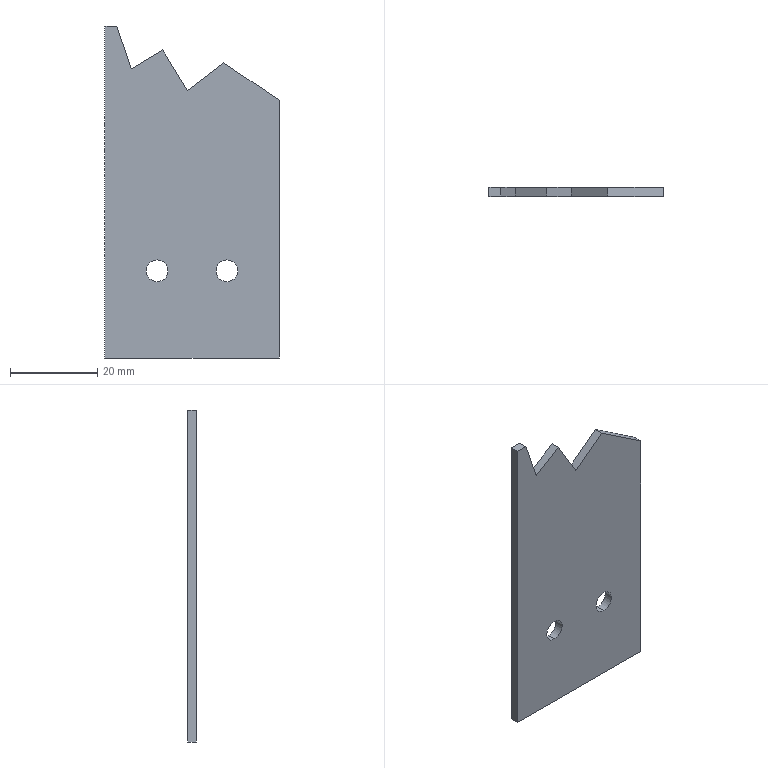Part | SolidWorks | features Cut 2, Extrusion 1 | 1 solid | 15 faces | box 40 x 2 x 76.221 mm | volume 5242 mm3 | plane 11 | cylinder 4 | commonest cylinder face diameters 5 x4
STEP:
#1=CARTESIAN_POINT('',(8.,2.,-22.5));
#2=VERTEX_POINT('',#1);
#3=CARTESIAN_POINT('',(8.,2.,-17.5));
#4=VERTEX_POINT('',#3);
#5=CARTESIAN_POINT('',(8.,2.,-20.));
#6=DIRECTION('',(0.,1.,0.));
#7=DIRECTION('',(0.,0.,1.));
#8=AXIS2_PLACEMENT_3D('',#5,#6,#7);
#9=CIRCLE('',#8,2.5);
#10=EDGE_CURVE('',#2,#4,#9,.T.);
#11=ORIENTED_EDGE('',*,*,#10,.T.);
#12=CARTESIAN_POINT('',(8.,0.,-17.5));
#13=VERTEX_POINT('',#12);
#14=CARTESIAN_POINT('',(8.,10.,-17.5));
#15=DIRECTION('',(0.,-1.,0.));
#16=VECTOR('',#15,1000.);
#17=LINE('',#14,#16);
#18=EDGE_CURVE('',#4,#13,#17,.T.);
#19=ORIENTED_EDGE('',*,*,#18,.T.);
#20=CARTESIAN_POINT('',(8.,0.,-22.5));
#21=VERTEX_POINT('',#20);
#22=CARTESIAN_POINT('',(8.,0.,-20.));
#23=DIRECTION('',(0.,-1.,0.));
#24=DIRECTION('',(0.,0.,-1.));
#25=AXIS2_PLACEMENT_3D('',#22,#23,#24);
#26=CIRCLE('',#25,2.5);
#27=EDGE_CURVE('',#13,#21,#26,.T.);
#28=ORIENTED_EDGE('',*,*,#27,.T.);
#29=CARTESIAN_POINT('',(8.,10.,-22.5));
#30=DIRECTION('',(0.,-1.,0.));
#31=VECTOR('',#30,1000.);
#32=LINE('',#29,#31);
#33=EDGE_CURVE('',#2,#21,#32,.T.);
#34=ORIENTED_EDGE('',*,*,#33,.F.);
#35=EDGE_LOOP('',(#11,#19,#28,#34));
#36=FACE_OUTER_BOUND('',#35,.T.);
#37=CARTESIAN_POINT('',(8.,10.,-20.));
#38=DIRECTION('',(0.,-1.,0.));
#39=DIRECTION('',(0.,0.,-1.));
#40=AXIS2_PLACEMENT_3D('',#37,#38,#39);
#41=CYLINDRICAL_SURFACE('',#40,2.5);
#42=ADVANCED_FACE('',(#36),#41,.F.);
#43=CARTESIAN_POINT('',(-8.,2.,-22.5));
#44=VERTEX_POINT('',#43);
#45=CARTESIAN_POINT('',(-8.,2.,-17.5));
#46=VERTEX_POINT('',#45);
#47=CARTESIAN_POINT('',(-8.,2.,-20.));
#48=DIRECTION('',(0.,1.,0.));
#49=DIRECTION('',(0.,0.,1.));
#50=AXIS2_PLACEMENT_3D('',#47,#48,#49);
#51=CIRCLE('',#50,2.5);
#52=EDGE_CURVE('',#44,#46,#51,.T.);
#53=ORIENTED_EDGE('',*,*,#52,.T.);
#54=CARTESIAN_POINT('',(-8.,0.,-17.5));
#55=VERTEX_POINT('',#54);
#56=CARTESIAN_POINT('',(-8.,10.,-17.5));
#57=DIRECTION('',(0.,-1.,0.));
#58=VECTOR('',#57,1000.);
#59=LINE('',#56,#58);
#60=EDGE_CURVE('',#46,#55,#59,.T.);
#61=ORIENTED_EDGE('',*,*,#60,.T.);
#62=CARTESIAN_POINT('',(-8.,0.,-22.5));
#63=VERTEX_POINT('',#62);
#64=CARTESIAN_POINT('',(-8.,0.,-20.));
#65=DIRECTION('',(0.,-1.,0.));
#66=DIRECTION('',(0.,0.,-1.));
#67=AXIS2_PLACEMENT_3D('',#64,#65,#66);
#68=CIRCLE('',#67,2.5);
#69=EDGE_CURVE('',#55,#63,#68,.T.);
#70=ORIENTED_EDGE('',*,*,#69,.T.);
#71=CARTESIAN_POINT('',(-8.,10.,-22.5));
#72=DIRECTION('',(0.,-1.,0.));
#73=VECTOR('',#72,1000.);
#74=LINE('',#71,#73);
#75=EDGE_CURVE('',#44,#63,#74,.T.);
#76=ORIENTED_EDGE('',*,*,#75,.F.);
#77=EDGE_LOOP('',(#53,#61,#70,#76));
#78=FACE_OUTER_BOUND('',#77,.T.);
#79=CARTESIAN_POINT('',(-8.,10.,-20.));
#80=DIRECTION('',(0.,-1.,0.));
#81=DIRECTION('',(0.,0.,-1.));
#82=AXIS2_PLACEMENT_3D('',#79,#80,#81);
#83=CYLINDRICAL_SURFACE('',#82,2.5);
#84=ADVANCED_FACE('',(#78),#83,.F.);
#85=CARTESIAN_POINT('',(20.,2.,19.198));
#86=VERTEX_POINT('',#85);
#87=CARTESIAN_POINT('',(20.,2.,-40.));
#88=VERTEX_POINT('',#87);
#89=CARTESIAN_POINT('',(20.,2.,-40.));
#90=DIRECTION('',(0.,0.,-1.));
#91=VECTOR('',#90,1000.);
#92=LINE('',#89,#91);
#93=EDGE_CURVE('',#86,#88,#92,.T.);
#94=ORIENTED_EDGE('',*,*,#93,.F.);
#95=CARTESIAN_POINT('',(20.,0.,19.198));
#96=VERTEX_POINT('',#95);
#97=CARTESIAN_POINT('',(20.,-8.,19.198));
#98=DIRECTION('',(0.,1.,0.));
#99=VECTOR('',#98,1000.);
#100=LINE('',#97,#99);
#101=EDGE_CURVE('',#96,#86,#100,.T.);
#102=ORIENTED_EDGE('',*,*,#101,.F.);
#103=CARTESIAN_POINT('',(20.,0.,-40.));
#104=VERTEX_POINT('',#103);
#105=CARTESIAN_POINT('',(20.,0.,-40.));
#106=DIRECTION('',(0.,0.,-1.));
#107=VECTOR('',#106,1000.);
#108=LINE('',#105,#107);
#109=EDGE_CURVE('',#96,#104,#108,.T.);
#110=ORIENTED_EDGE('',*,*,#109,.T.);
#111=CARTESIAN_POINT('',(20.,2.,-40.));
#112=DIRECTION('',(0.,-1.,0.));
#113=VECTOR('',#112,1000.);
#114=LINE('',#111,#113);
#115=EDGE_CURVE('',#88,#104,#114,.T.);
#116=ORIENTED_EDGE('',*,*,#115,.F.);
#117=EDGE_LOOP('',(#94,#102,#110,#116));
#118=FACE_OUTER_BOUND('',#117,.T.);
#119=CARTESIAN_POINT('',(20.,2.,-40.));
#120=DIRECTION('',(-1.,0.,0.));
#121=DIRECTION('',(0.,0.,1.));
#122=AXIS2_PLACEMENT_3D('',#119,#120,#121);
#123=PLANE('',#122);
#124=ADVANCED_FACE('',(#118),#123,.F.);
#125=CARTESIAN_POINT('',(-20.,0.,-40.));
#126=VERTEX_POINT('',#125);
#127=CARTESIAN_POINT('',(-20.,0.,-40.));
#128=DIRECTION('',(-1.,0.,0.));
#129=VECTOR('',#128,1000.);
#130=LINE('',#127,#129);
#131=EDGE_CURVE('',#104,#126,#130,.T.);
#132=ORIENTED_EDGE('',*,*,#131,.T.);
#133=CARTESIAN_POINT('',(-20.,2.,-40.));
#134=VERTEX_POINT('',#133);
#135=CARTESIAN_POINT('',(-20.,2.,-40.));
#136=DIRECTION('',(0.,-1.,0.));
#137=VECTOR('',#136,1000.);
#138=LINE('',#135,#137);
#139=EDGE_CURVE('',#134,#126,#138,.T.);
#140=ORIENTED_EDGE('',*,*,#139,.F.);
#141=CARTESIAN_POINT('',(-20.,2.,-40.));
#142=DIRECTION('',(-1.,0.,0.));
#143=VECTOR('',#142,1000.);
#144=LINE('',#141,#143);
#145=EDGE_CURVE('',#88,#134,#144,.T.);
#146=ORIENTED_EDGE('',*,*,#145,.F.);
#147=ORIENTED_EDGE('',*,*,#115,.T.);
#148=EDGE_LOOP('',(#132,#140,#146,#147));
#149=FACE_OUTER_BOUND('',#148,.T.);
#150=CARTESIAN_POINT('',(-20.,2.,-40.));
#151=DIRECTION('',(0.,0.,1.));
#152=DIRECTION('',(1.,0.,0.));
#153=AXIS2_PLACEMENT_3D('',#150,#151,#152);
#154=PLANE('',#153);
#155=ADVANCED_FACE('',(#149),#154,.F.);
#156=CARTESIAN_POINT('',(-20.,0.,36.221));
#157=VERTEX_POINT('',#156);
#158=CARTESIAN_POINT('',(-20.,0.,-40.));
#159=DIRECTION('',(0.,0.,1.));
#160=VECTOR('',#159,1000.);
#161=LINE('',#158,#160);
#162=EDGE_CURVE('',#126,#157,#161,.T.);
#163=ORIENTED_EDGE('',*,*,#162,.T.);
#164=CARTESIAN_POINT('',(-20.,2.,36.221));
#165=VERTEX_POINT('',#164);
#166=CARTESIAN_POINT('',(-20.,-8.,36.221));
#167=DIRECTION('',(0.,1.,0.));
#168=VECTOR('',#167,1000.);
#169=LINE('',#166,#168);
#170=EDGE_CURVE('',#157,#165,#169,.T.);
#171=ORIENTED_EDGE('',*,*,#170,.T.);
#172=CARTESIAN_POINT('',(-20.,2.,-40.));
#173=DIRECTION('',(0.,0.,1.));
#174=VECTOR('',#173,1000.);
#175=LINE('',#172,#174);
#176=EDGE_CURVE('',#134,#165,#175,.T.);
#177=ORIENTED_EDGE('',*,*,#176,.F.);
#178=ORIENTED_EDGE('',*,*,#139,.T.);
#179=EDGE_LOOP('',(#163,#171,#177,#178));
#180=FACE_OUTER_BOUND('',#179,.T.);
#181=CARTESIAN_POINT('',(-20.,2.,-40.));
#182=DIRECTION('',(1.,0.,0.));
#183=DIRECTION('',(0.,0.,-1.));
#184=AXIS2_PLACEMENT_3D('',#181,#182,#183);
#185=PLANE('',#184);
#186=ADVANCED_FACE('',(#180),#185,.F.);
#187=CARTESIAN_POINT('',(-17.266,2.,36.221));
#188=VERTEX_POINT('',#187);
#189=CARTESIAN_POINT('',(-17.266,2.,36.221));
#190=DIRECTION('',(-1.,0.,0.));
#191=VECTOR('',#190,1000.);
#192=LINE('',#189,#191);
#193=EDGE_CURVE('',#188,#165,#192,.T.);
#194=ORIENTED_EDGE('',*,*,#193,.F.);
#195=CARTESIAN_POINT('',(-13.941,2.,26.358));
#196=VERTEX_POINT('',#195);
#197=CARTESIAN_POINT('',(-13.941,2.,26.358));
#198=DIRECTION('',(-0.3194,0.,0.9476));
#199=VECTOR('',#198,1000.);
#200=LINE('',#197,#199);
#201=EDGE_CURVE('',#196,#188,#200,.T.);
#202=ORIENTED_EDGE('',*,*,#201,.F.);
#203=CARTESIAN_POINT('',(-6.728,2.,30.727));
#204=VERTEX_POINT('',#203);
#205=CARTESIAN_POINT('',(-6.728,2.,30.727));
#206=DIRECTION('',(-0.8553,0.,-0.5181));
#207=VECTOR('',#206,1000.);
#208=LINE('',#205,#207);
#209=EDGE_CURVE('',#204,#196,#208,.T.);
#210=ORIENTED_EDGE('',*,*,#209,.F.);
#211=CARTESIAN_POINT('',(-1.054,2.,21.36));
#212=VERTEX_POINT('',#211);
#213=CARTESIAN_POINT('',(-1.054,2.,21.36));
#214=DIRECTION('',(-0.5181,0.,0.8553));
#215=VECTOR('',#214,1000.);
#216=LINE('',#213,#215);
#217=EDGE_CURVE('',#212,#204,#216,.T.);
#218=ORIENTED_EDGE('',*,*,#217,.F.);
#219=CARTESIAN_POINT('',(7.323,2.,27.755));
#220=VERTEX_POINT('',#219);
#221=CARTESIAN_POINT('',(7.323,2.,27.755));
#222=DIRECTION('',(-0.7948,0.,-0.6068));
#223=VECTOR('',#222,1000.);
#224=LINE('',#221,#223);
#225=EDGE_CURVE('',#220,#212,#224,.T.);
#226=ORIENTED_EDGE('',*,*,#225,.F.);
#227=CARTESIAN_POINT('',(20.,2.,19.198));
#228=DIRECTION('',(-0.8289,0.,0.5595));
#229=VECTOR('',#228,1000.);
#230=LINE('',#227,#229);
#231=EDGE_CURVE('',#86,#220,#230,.T.);
#232=ORIENTED_EDGE('',*,*,#231,.F.);
#233=ORIENTED_EDGE('',*,*,#93,.T.);
#234=ORIENTED_EDGE('',*,*,#145,.T.);
#235=ORIENTED_EDGE('',*,*,#176,.T.);
#236=EDGE_LOOP('',(#194,#202,#210,#218,#226,#232,#233,#234,#235));
#237=FACE_OUTER_BOUND('',#236,.T.);
#238=ORIENTED_EDGE('',*,*,#10,.F.);
#239=CARTESIAN_POINT('',(8.,2.,-20.));
#240=DIRECTION('',(0.,1.,0.));
#241=DIRECTION('',(0.,0.,1.));
#242=AXIS2_PLACEMENT_3D('',#239,#240,#241);
#243=CIRCLE('',#242,2.5);
#244=EDGE_CURVE('',#4,#2,#243,.T.);
#245=ORIENTED_EDGE('',*,*,#244,.F.);
#246=EDGE_LOOP('',(#238,#245));
#247=FACE_BOUND('',#246,.T.);
#248=ORIENTED_EDGE('',*,*,#52,.F.);
#249=CARTESIAN_POINT('',(-8.,2.,-20.));
#250=DIRECTION('',(0.,1.,0.));
#251=DIRECTION('',(0.,0.,1.));
#252=AXIS2_PLACEMENT_3D('',#249,#250,#251);
#253=CIRCLE('',#252,2.5);
#254=EDGE_CURVE('',#46,#44,#253,.T.);
#255=ORIENTED_EDGE('',*,*,#254,.F.);
#256=EDGE_LOOP('',(#248,#255));
#257=FACE_BOUND('',#256,.T.);
#258=CARTESIAN_POINT('',(0.,2.,0.));
#259=DIRECTION('',(0.,1.,0.));
#260=DIRECTION('',(0.,0.,1.));
#261=AXIS2_PLACEMENT_3D('',#258,#259,#260);
#262=PLANE('',#261);
#263=ADVANCED_FACE('',(#237,#247,#257),#262,.T.);
#264=CARTESIAN_POINT('',(8.,0.,-20.));
#265=DIRECTION('',(0.,-1.,0.));
#266=DIRECTION('',(0.,0.,-1.));
#267=AXIS2_PLACEMENT_3D('',#264,#265,#266);
#268=CIRCLE('',#267,2.5);
#269=EDGE_CURVE('',#21,#13,#268,.T.);
#270=ORIENTED_EDGE('',*,*,#269,.F.);
#271=ORIENTED_EDGE('',*,*,#27,.F.);
#272=EDGE_LOOP('',(#270,#271));
#273=FACE_BOUND('',#272,.T.);
#274=CARTESIAN_POINT('',(-8.,0.,-20.));
#275=DIRECTION('',(0.,-1.,0.));
#276=DIRECTION('',(0.,0.,-1.));
#277=AXIS2_PLACEMENT_3D('',#274,#275,#276);
#278=CIRCLE('',#277,2.5);
#279=EDGE_CURVE('',#63,#55,#278,.T.);
#280=ORIENTED_EDGE('',*,*,#279,.F.);
#281=ORIENTED_EDGE('',*,*,#69,.F.);
#282=EDGE_LOOP('',(#280,#281));
#283=FACE_BOUND('',#282,.T.);
#284=CARTESIAN_POINT('',(-13.941,0.,26.358));
#285=VERTEX_POINT('',#284);
#286=CARTESIAN_POINT('',(-17.266,0.,36.221));
#287=VERTEX_POINT('',#286);
#288=CARTESIAN_POINT('',(-4.54,0.,-1.53));
#289=DIRECTION('',(-0.3194,0.,0.9476));
#290=VECTOR('',#289,1000.);
#291=LINE('',#288,#290);
#292=EDGE_CURVE('',#285,#287,#291,.T.);
#293=ORIENTED_EDGE('',*,*,#292,.T.);
#294=CARTESIAN_POINT('',(0.,0.,36.221));
#295=DIRECTION('',(-1.,0.,0.));
#296=VECTOR('',#295,1000.);
#297=LINE('',#294,#296);
#298=EDGE_CURVE('',#287,#157,#297,.T.);
#299=ORIENTED_EDGE('',*,*,#298,.T.);
#300=ORIENTED_EDGE('',*,*,#162,.F.);
#301=ORIENTED_EDGE('',*,*,#131,.F.);
#302=ORIENTED_EDGE('',*,*,#109,.F.);
#303=CARTESIAN_POINT('',(7.323,0.,27.755));
#304=VERTEX_POINT('',#303);
#305=CARTESIAN_POINT('',(15.162,0.,22.464));
#306=DIRECTION('',(-0.8289,0.,0.5595));
#307=VECTOR('',#306,1000.);
#308=LINE('',#305,#307);
#309=EDGE_CURVE('',#96,#304,#308,.T.);
#310=ORIENTED_EDGE('',*,*,#309,.T.);
#311=CARTESIAN_POINT('',(-1.054,0.,21.36));
#312=VERTEX_POINT('',#311);
#313=CARTESIAN_POINT('',(-10.69,0.,14.003));
#314=DIRECTION('',(-0.7948,0.,-0.6068));
#315=VECTOR('',#314,1000.);
#316=LINE('',#313,#315);
#317=EDGE_CURVE('',#304,#312,#316,.T.);
#318=ORIENTED_EDGE('',*,*,#317,.T.);
#319=CARTESIAN_POINT('',(-6.728,0.,30.727));
#320=VERTEX_POINT('',#319);
#321=CARTESIAN_POINT('',(8.695,0.,5.267));
#322=DIRECTION('',(-0.5181,0.,0.8553));
#323=VECTOR('',#322,1000.);
#324=LINE('',#321,#323);
#325=EDGE_CURVE('',#312,#320,#324,.T.);
#326=ORIENTED_EDGE('',*,*,#325,.T.);
#327=CARTESIAN_POINT('',(-15.423,0.,25.46));
#328=DIRECTION('',(-0.8553,0.,-0.5181));
#329=VECTOR('',#328,1000.);
#330=LINE('',#327,#329);
#331=EDGE_CURVE('',#320,#285,#330,.T.);
#332=ORIENTED_EDGE('',*,*,#331,.T.);
#333=EDGE_LOOP('',(#293,#299,#300,#301,#302,#310,#318,#326,#332));
#334=FACE_OUTER_BOUND('',#333,.T.);
#335=CARTESIAN_POINT('',(0.,0.,0.));
#336=DIRECTION('',(0.,1.,0.));
#337=DIRECTION('',(0.,0.,1.));
#338=AXIS2_PLACEMENT_3D('',#335,#336,#337);
#339=PLANE('',#338);
#340=ADVANCED_FACE('',(#273,#283,#334),#339,.F.);
#341=ORIENTED_EDGE('',*,*,#60,.F.);
#342=ORIENTED_EDGE('',*,*,#254,.T.);
#343=ORIENTED_EDGE('',*,*,#75,.T.);
#344=ORIENTED_EDGE('',*,*,#279,.T.);
#345=EDGE_LOOP('',(#341,#342,#343,#344));
#346=FACE_OUTER_BOUND('',#345,.T.);
#347=CARTESIAN_POINT('',(-8.,10.,-20.));
#348=DIRECTION('',(0.,-1.,0.));
#349=DIRECTION('',(0.,0.,-1.));
#350=AXIS2_PLACEMENT_3D('',#347,#348,#349);
#351=CYLINDRICAL_SURFACE('',#350,2.5);
#352=ADVANCED_FACE('',(#346),#351,.F.);
#353=ORIENTED_EDGE('',*,*,#18,.F.);
#354=ORIENTED_EDGE('',*,*,#244,.T.);
#355=ORIENTED_EDGE('',*,*,#33,.T.);
#356=ORIENTED_EDGE('',*,*,#269,.T.);
#357=EDGE_LOOP('',(#353,#354,#355,#356));
#358=FACE_OUTER_BOUND('',#357,.T.);
#359=CARTESIAN_POINT('',(8.,10.,-20.));
#360=DIRECTION('',(0.,-1.,0.));
#361=DIRECTION('',(0.,0.,-1.));
#362=AXIS2_PLACEMENT_3D('',#359,#360,#361);
#363=CYLINDRICAL_SURFACE('',#362,2.5);
#364=ADVANCED_FACE('',(#358),#363,.F.);
#365=CARTESIAN_POINT('',(-17.266,-8.,36.221));
#366=DIRECTION('',(0.,1.,0.));
#367=VECTOR('',#366,1000.);
#368=LINE('',#365,#367);
#369=EDGE_CURVE('',#287,#188,#368,.T.);
#370=ORIENTED_EDGE('',*,*,#369,.T.);
#371=ORIENTED_EDGE('',*,*,#193,.T.);
#372=ORIENTED_EDGE('',*,*,#170,.F.);
#373=ORIENTED_EDGE('',*,*,#298,.F.);
#374=EDGE_LOOP('',(#370,#371,#372,#373));
#375=FACE_OUTER_BOUND('',#374,.T.);
#376=CARTESIAN_POINT('',(-17.266,-8.,36.221));
#377=DIRECTION('',(0.,0.,-1.));
#378=DIRECTION('',(-1.,0.,0.));
#379=AXIS2_PLACEMENT_3D('',#376,#377,#378);
#380=PLANE('',#379);
#381=ADVANCED_FACE('',(#375),#380,.F.);
#382=CARTESIAN_POINT('',(-13.941,-8.,26.358));
#383=DIRECTION('',(0.,1.,0.));
#384=VECTOR('',#383,1000.);
#385=LINE('',#382,#384);
#386=EDGE_CURVE('',#285,#196,#385,.T.);
#387=ORIENTED_EDGE('',*,*,#386,.T.);
#388=ORIENTED_EDGE('',*,*,#201,.T.);
#389=ORIENTED_EDGE('',*,*,#369,.F.);
#390=ORIENTED_EDGE('',*,*,#292,.F.);
#391=EDGE_LOOP('',(#387,#388,#389,#390));
#392=FACE_OUTER_BOUND('',#391,.T.);
#393=CARTESIAN_POINT('',(-13.941,-8.,26.358));
#394=DIRECTION('',(-0.9476,0.,-0.3194));
#395=DIRECTION('',(-0.3194,0.,0.9476));
#396=AXIS2_PLACEMENT_3D('',#393,#394,#395);
#397=PLANE('',#396);
#398=ADVANCED_FACE('',(#392),#397,.F.);
#399=CARTESIAN_POINT('',(-6.728,-8.,30.727));
#400=DIRECTION('',(0.,1.,0.));
#401=VECTOR('',#400,1000.);
#402=LINE('',#399,#401);
#403=EDGE_CURVE('',#320,#204,#402,.T.);
#404=ORIENTED_EDGE('',*,*,#403,.T.);
#405=ORIENTED_EDGE('',*,*,#209,.T.);
#406=ORIENTED_EDGE('',*,*,#386,.F.);
#407=ORIENTED_EDGE('',*,*,#331,.F.);
#408=EDGE_LOOP('',(#404,#405,#406,#407));
#409=FACE_OUTER_BOUND('',#408,.T.);
#410=CARTESIAN_POINT('',(-6.728,-8.,30.727));
#411=DIRECTION('',(0.5181,0.,-0.8553));
#412=DIRECTION('',(-0.8553,0.,-0.5181));
#413=AXIS2_PLACEMENT_3D('',#410,#411,#412);
#414=PLANE('',#413);
#415=ADVANCED_FACE('',(#409),#414,.F.);
#416=CARTESIAN_POINT('',(-1.054,-8.,21.36));
#417=DIRECTION('',(0.,1.,0.));
#418=VECTOR('',#417,1000.);
#419=LINE('',#416,#418);
#420=EDGE_CURVE('',#312,#212,#419,.T.);
#421=ORIENTED_EDGE('',*,*,#420,.T.);
#422=ORIENTED_EDGE('',*,*,#217,.T.);
#423=ORIENTED_EDGE('',*,*,#403,.F.);
#424=ORIENTED_EDGE('',*,*,#325,.F.);
#425=EDGE_LOOP('',(#421,#422,#423,#424));
#426=FACE_OUTER_BOUND('',#425,.T.);
#427=CARTESIAN_POINT('',(-1.054,-8.,21.36));
#428=DIRECTION('',(-0.8553,0.,-0.5181));
#429=DIRECTION('',(-0.5181,0.,0.8553));
#430=AXIS2_PLACEMENT_3D('',#427,#428,#429);
#431=PLANE('',#430);
#432=ADVANCED_FACE('',(#426),#431,.F.);
#433=CARTESIAN_POINT('',(7.323,-8.,27.755));
#434=DIRECTION('',(0.,1.,0.));
#435=VECTOR('',#434,1000.);
#436=LINE('',#433,#435);
#437=EDGE_CURVE('',#304,#220,#436,.T.);
#438=ORIENTED_EDGE('',*,*,#437,.T.);
#439=ORIENTED_EDGE('',*,*,#225,.T.);
#440=ORIENTED_EDGE('',*,*,#420,.F.);
#441=ORIENTED_EDGE('',*,*,#317,.F.);
#442=EDGE_LOOP('',(#438,#439,#440,#441));
#443=FACE_OUTER_BOUND('',#442,.T.);
#444=CARTESIAN_POINT('',(7.323,-8.,27.755));
#445=DIRECTION('',(0.6068,0.,-0.7948));
#446=DIRECTION('',(-0.7948,0.,-0.6068));
#447=AXIS2_PLACEMENT_3D('',#444,#445,#446);
#448=PLANE('',#447);
#449=ADVANCED_FACE('',(#443),#448,.F.);
#450=ORIENTED_EDGE('',*,*,#101,.T.);
#451=ORIENTED_EDGE('',*,*,#231,.T.);
#452=ORIENTED_EDGE('',*,*,#437,.F.);
#453=ORIENTED_EDGE('',*,*,#309,.F.);
#454=EDGE_LOOP('',(#450,#451,#452,#453));
#455=FACE_OUTER_BOUND('',#454,.T.);
#456=CARTESIAN_POINT('',(20.,-8.,19.198));
#457=DIRECTION('',(-0.5595,0.,-0.8289));
#458=DIRECTION('',(-0.8289,0.,0.5595));
#459=AXIS2_PLACEMENT_3D('',#456,#457,#458);
#460=PLANE('',#459);
#461=ADVANCED_FACE('',(#455),#460,.F.);
#462=CLOSED_SHELL('',(#42,#84,#124,#155,#186,#263,#340,#352,#364,#381,#398,#415,#432,#449,#461));
#463=MANIFOLD_SOLID_BREP('',#462);
#464=CARTESIAN_POINT('',(0.,0.,0.));
#465=DIRECTION('',(0.,0.,1.));
#466=DIRECTION('',(1.,0.,0.));
#467=AXIS2_PLACEMENT_3D('',#464,#465,#466);
#468=(LENGTH_UNIT()NAMED_UNIT(*)SI_UNIT(.MILLI.,.METRE.));
#469=UNCERTAINTY_MEASURE_WITH_UNIT(LENGTH_MEASURE(0.00001),#468,'','');
#470=(NAMED_UNIT(*)PLANE_ANGLE_UNIT()SI_UNIT($,.RADIAN.));
#471=(NAMED_UNIT(*)SI_UNIT($,.STERADIAN.)SOLID_ANGLE_UNIT());
#472=(GEOMETRIC_REPRESENTATION_CONTEXT(3)GLOBAL_UNCERTAINTY_ASSIGNED_CONTEXT((#469))GLOBAL_UNIT_ASSIGNED_CONTEXT((#468,#470,#471))REPRESENTATION_CONTEXT('',''));
#473=ADVANCED_BREP_SHAPE_REPRESENTATION('',(#463,#467),#472);